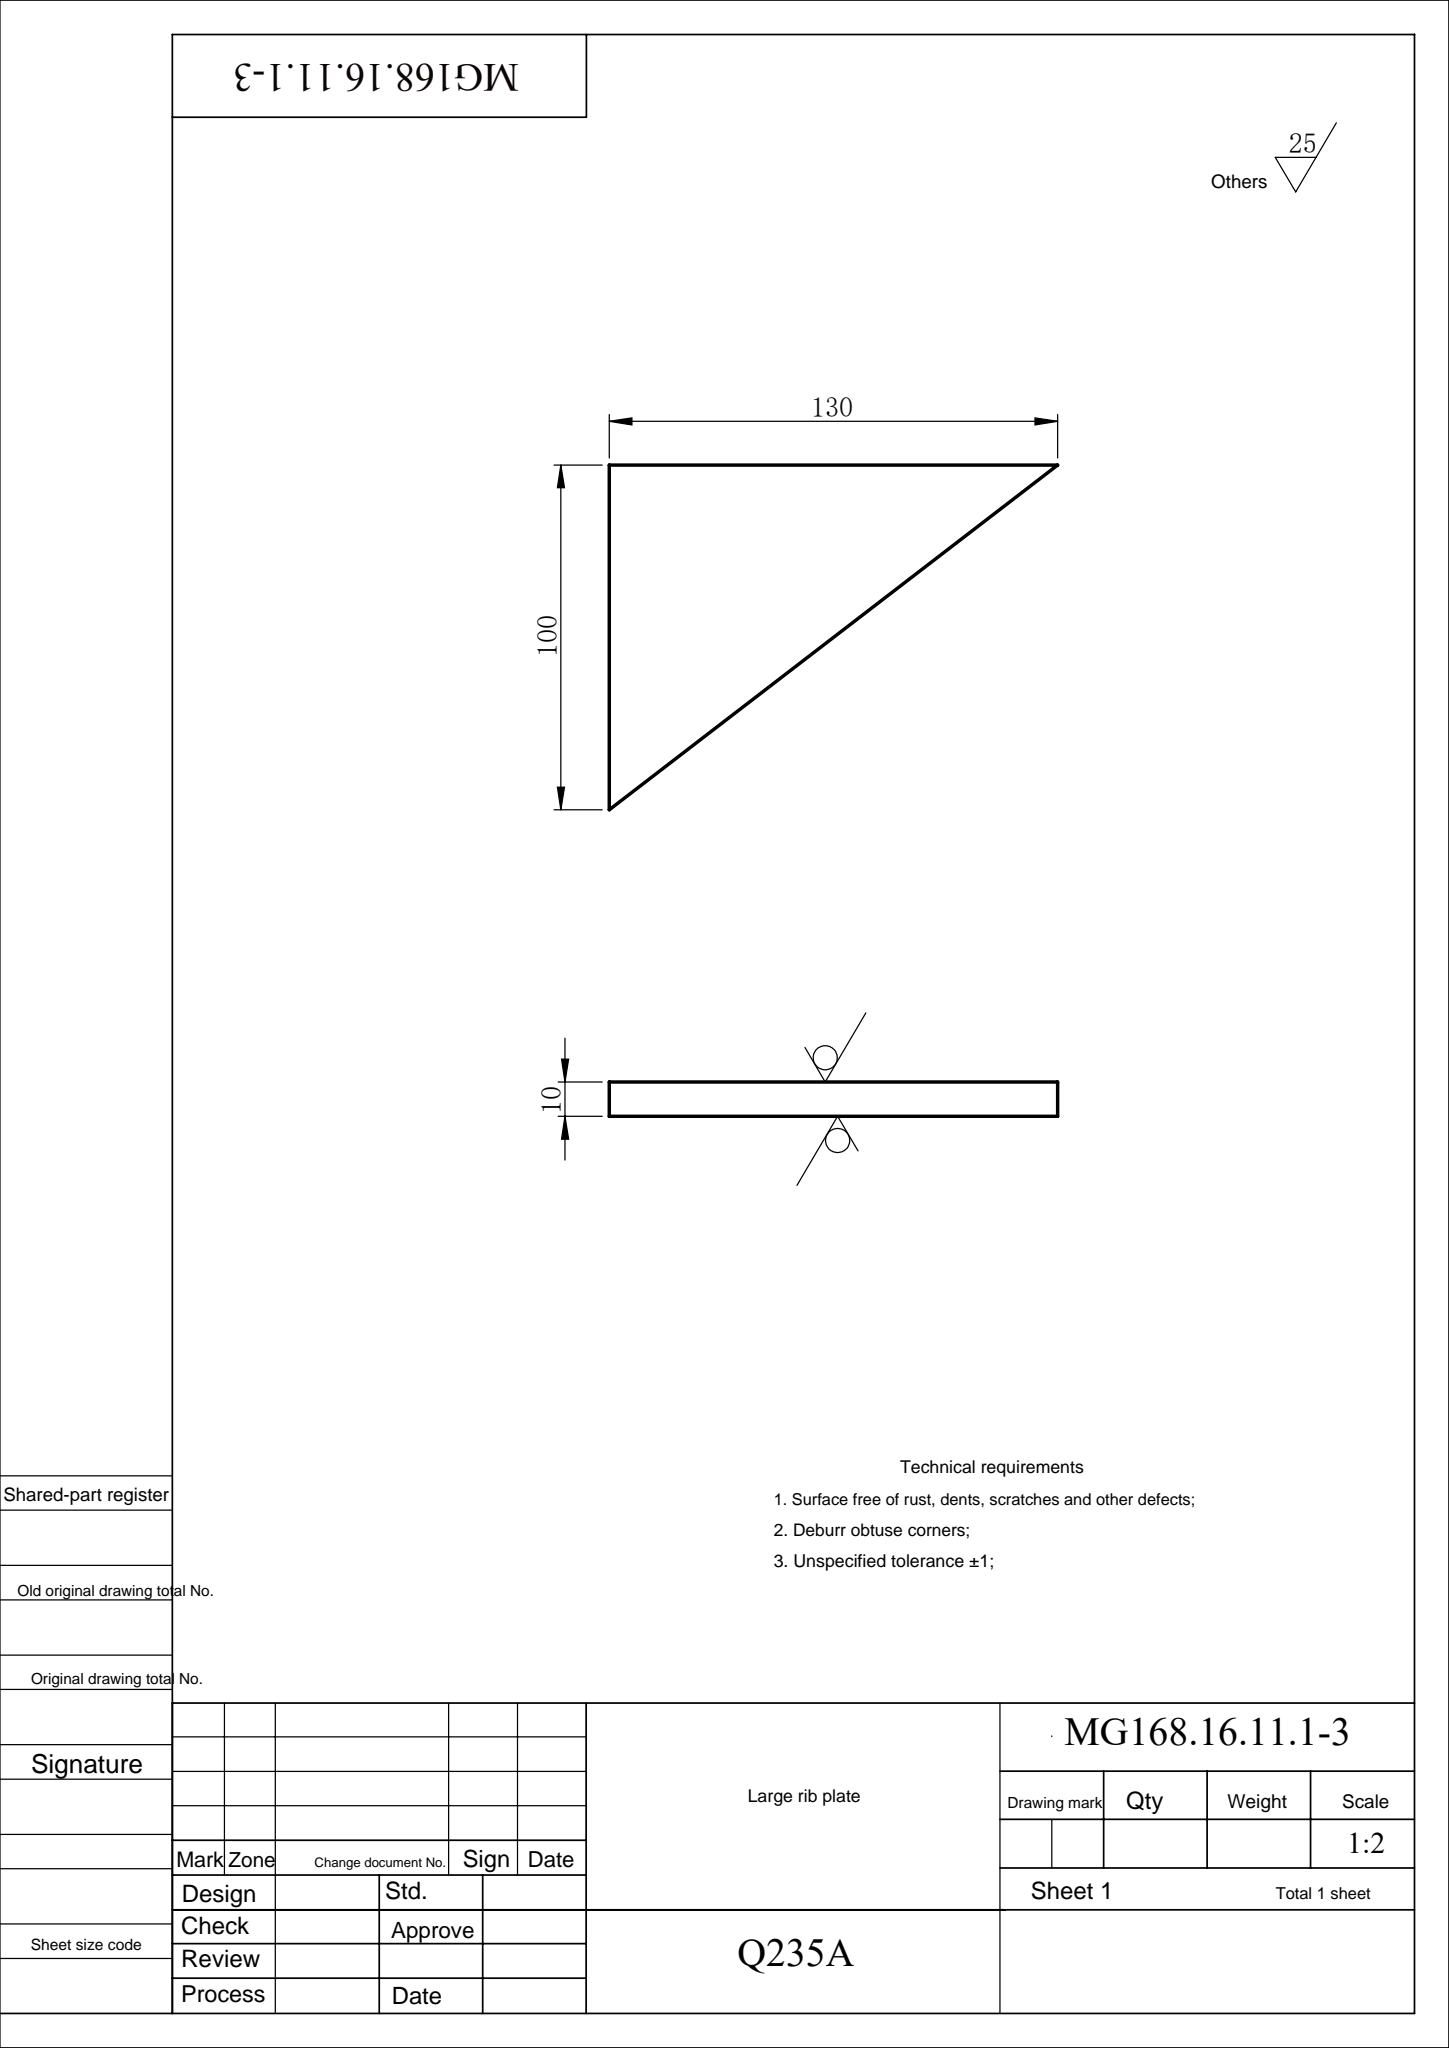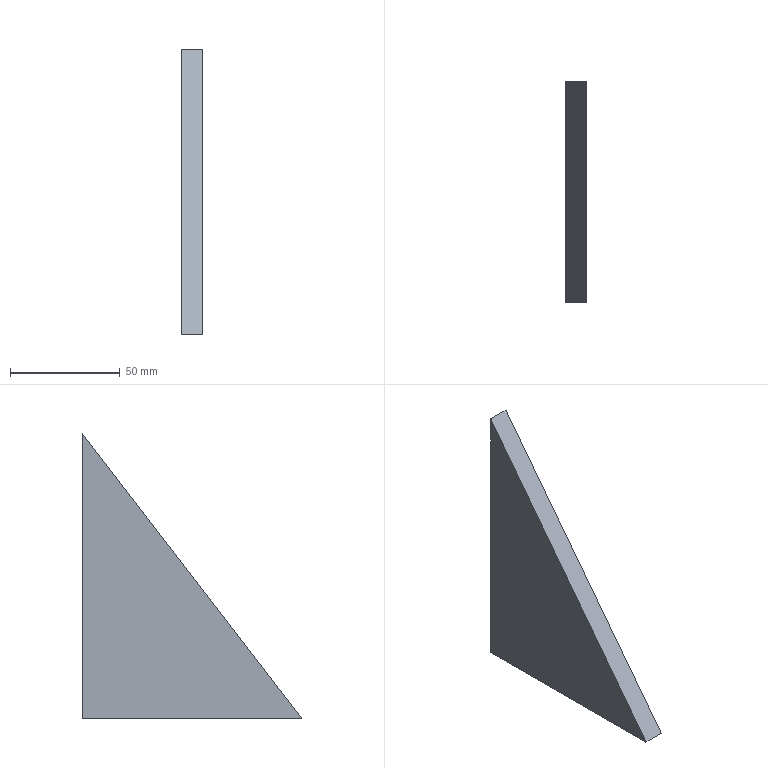Part | SolidWorks | features Extrusion 1 | 1 solid | 5 faces | box 10 x 100 x 130 mm | volume 65000 mm3 | plane 5
STEP:
#1=CARTESIAN_POINT('',(-5.,0.,130.));
#2=VERTEX_POINT('',#1);
#3=CARTESIAN_POINT('',(-5.,-100.,0.));
#4=VERTEX_POINT('',#3);
#5=CARTESIAN_POINT('',(-5.,-100.,0.));
#6=DIRECTION('',(0.,-0.6097,-0.7926));
#7=VECTOR('',#6,1000.);
#8=LINE('',#5,#7);
#9=EDGE_CURVE('',#2,#4,#8,.T.);
#10=ORIENTED_EDGE('',*,*,#9,.T.);
#11=CARTESIAN_POINT('',(5.,-100.,0.));
#12=VERTEX_POINT('',#11);
#13=CARTESIAN_POINT('',(5.,-100.,0.));
#14=DIRECTION('',(-1.,0.,0.));
#15=VECTOR('',#14,1000.);
#16=LINE('',#13,#15);
#17=EDGE_CURVE('',#12,#4,#16,.T.);
#18=ORIENTED_EDGE('',*,*,#17,.F.);
#19=CARTESIAN_POINT('',(5.,0.,130.));
#20=VERTEX_POINT('',#19);
#21=CARTESIAN_POINT('',(5.,-100.,0.));
#22=DIRECTION('',(0.,-0.6097,-0.7926));
#23=VECTOR('',#22,1000.);
#24=LINE('',#21,#23);
#25=EDGE_CURVE('',#20,#12,#24,.T.);
#26=ORIENTED_EDGE('',*,*,#25,.F.);
#27=CARTESIAN_POINT('',(5.,0.,130.));
#28=DIRECTION('',(-1.,0.,0.));
#29=VECTOR('',#28,1000.);
#30=LINE('',#27,#29);
#31=EDGE_CURVE('',#20,#2,#30,.T.);
#32=ORIENTED_EDGE('',*,*,#31,.T.);
#33=EDGE_LOOP('',(#10,#18,#26,#32));
#34=FACE_OUTER_BOUND('',#33,.T.);
#35=CARTESIAN_POINT('',(5.,-100.,0.));
#36=DIRECTION('',(0.,0.7926,-0.6097));
#37=DIRECTION('',(0.,0.6097,0.7926));
#38=AXIS2_PLACEMENT_3D('',#35,#36,#37);
#39=PLANE('',#38);
#40=ADVANCED_FACE('',(#34),#39,.F.);
#41=CARTESIAN_POINT('',(-5.,0.,0.));
#42=VERTEX_POINT('',#41);
#43=CARTESIAN_POINT('',(-5.,0.,0.));
#44=DIRECTION('',(0.,1.,0.));
#45=VECTOR('',#44,1000.);
#46=LINE('',#43,#45);
#47=EDGE_CURVE('',#4,#42,#46,.T.);
#48=ORIENTED_EDGE('',*,*,#47,.T.);
#49=CARTESIAN_POINT('',(5.,0.,0.));
#50=VERTEX_POINT('',#49);
#51=CARTESIAN_POINT('',(5.,0.,0.));
#52=DIRECTION('',(-1.,0.,0.));
#53=VECTOR('',#52,1000.);
#54=LINE('',#51,#53);
#55=EDGE_CURVE('',#50,#42,#54,.T.);
#56=ORIENTED_EDGE('',*,*,#55,.F.);
#57=CARTESIAN_POINT('',(5.,0.,0.));
#58=DIRECTION('',(0.,1.,0.));
#59=VECTOR('',#58,1000.);
#60=LINE('',#57,#59);
#61=EDGE_CURVE('',#12,#50,#60,.T.);
#62=ORIENTED_EDGE('',*,*,#61,.F.);
#63=ORIENTED_EDGE('',*,*,#17,.T.);
#64=EDGE_LOOP('',(#48,#56,#62,#63));
#65=FACE_OUTER_BOUND('',#64,.T.);
#66=CARTESIAN_POINT('',(5.,0.,0.));
#67=DIRECTION('',(0.,0.,1.));
#68=DIRECTION('',(0.,-1.,0.));
#69=AXIS2_PLACEMENT_3D('',#66,#67,#68);
#70=PLANE('',#69);
#71=ADVANCED_FACE('',(#65),#70,.F.);
#72=CARTESIAN_POINT('',(-5.,0.,130.));
#73=DIRECTION('',(0.,0.,1.));
#74=VECTOR('',#73,1000.);
#75=LINE('',#72,#74);
#76=EDGE_CURVE('',#42,#2,#75,.T.);
#77=ORIENTED_EDGE('',*,*,#76,.T.);
#78=ORIENTED_EDGE('',*,*,#31,.F.);
#79=CARTESIAN_POINT('',(5.,0.,130.));
#80=DIRECTION('',(0.,0.,1.));
#81=VECTOR('',#80,1000.);
#82=LINE('',#79,#81);
#83=EDGE_CURVE('',#50,#20,#82,.T.);
#84=ORIENTED_EDGE('',*,*,#83,.F.);
#85=ORIENTED_EDGE('',*,*,#55,.T.);
#86=EDGE_LOOP('',(#77,#78,#84,#85));
#87=FACE_OUTER_BOUND('',#86,.T.);
#88=CARTESIAN_POINT('',(5.,0.,130.));
#89=DIRECTION('',(0.,-1.,0.));
#90=DIRECTION('',(0.,0.,-1.));
#91=AXIS2_PLACEMENT_3D('',#88,#89,#90);
#92=PLANE('',#91);
#93=ADVANCED_FACE('',(#87),#92,.F.);
#94=ORIENTED_EDGE('',*,*,#25,.T.);
#95=ORIENTED_EDGE('',*,*,#61,.T.);
#96=ORIENTED_EDGE('',*,*,#83,.T.);
#97=EDGE_LOOP('',(#94,#95,#96));
#98=FACE_OUTER_BOUND('',#97,.T.);
#99=CARTESIAN_POINT('',(5.,0.,0.));
#100=DIRECTION('',(1.,0.,0.));
#101=DIRECTION('',(0.,0.,-1.));
#102=AXIS2_PLACEMENT_3D('',#99,#100,#101);
#103=PLANE('',#102);
#104=ADVANCED_FACE('',(#98),#103,.T.);
#105=ORIENTED_EDGE('',*,*,#9,.F.);
#106=ORIENTED_EDGE('',*,*,#76,.F.);
#107=ORIENTED_EDGE('',*,*,#47,.F.);
#108=EDGE_LOOP('',(#105,#106,#107));
#109=FACE_OUTER_BOUND('',#108,.T.);
#110=CARTESIAN_POINT('',(-5.,0.,0.));
#111=DIRECTION('',(1.,0.,0.));
#112=DIRECTION('',(0.,0.,-1.));
#113=AXIS2_PLACEMENT_3D('',#110,#111,#112);
#114=PLANE('',#113);
#115=ADVANCED_FACE('',(#109),#114,.F.);
#116=CLOSED_SHELL('',(#40,#71,#93,#104,#115));
#117=MANIFOLD_SOLID_BREP('',#116);
#118=CARTESIAN_POINT('',(0.,0.,0.));
#119=DIRECTION('',(0.,0.,1.));
#120=DIRECTION('',(1.,0.,0.));
#121=AXIS2_PLACEMENT_3D('',#118,#119,#120);
#122=(LENGTH_UNIT()NAMED_UNIT(*)SI_UNIT(.MILLI.,.METRE.));
#123=UNCERTAINTY_MEASURE_WITH_UNIT(LENGTH_MEASURE(0.00001),#122,'','');
#124=(NAMED_UNIT(*)PLANE_ANGLE_UNIT()SI_UNIT($,.RADIAN.));
#125=(NAMED_UNIT(*)SI_UNIT($,.STERADIAN.)SOLID_ANGLE_UNIT());
#126=(GEOMETRIC_REPRESENTATION_CONTEXT(3)GLOBAL_UNCERTAINTY_ASSIGNED_CONTEXT((#123))GLOBAL_UNIT_ASSIGNED_CONTEXT((#122,#124,#125))REPRESENTATION_CONTEXT('',''));
#127=ADVANCED_BREP_SHAPE_REPRESENTATION('',(#117,#121),#126);